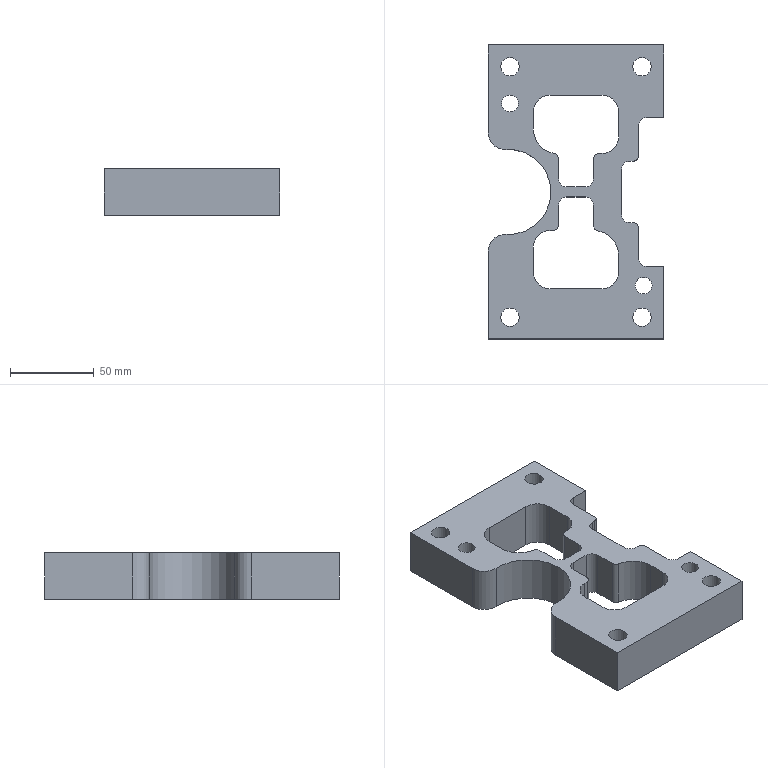Part | STEP file | PN_0022_id1018_x_t | 1 solid | 68 faces | box 105 x 176 x 28 mm | volume 281247 mm3 | cylinder 35 | plane 33 | commonest cylinder face diameters 10 x10 20 x8 6 x6 11 x4 17 x4 30 x2